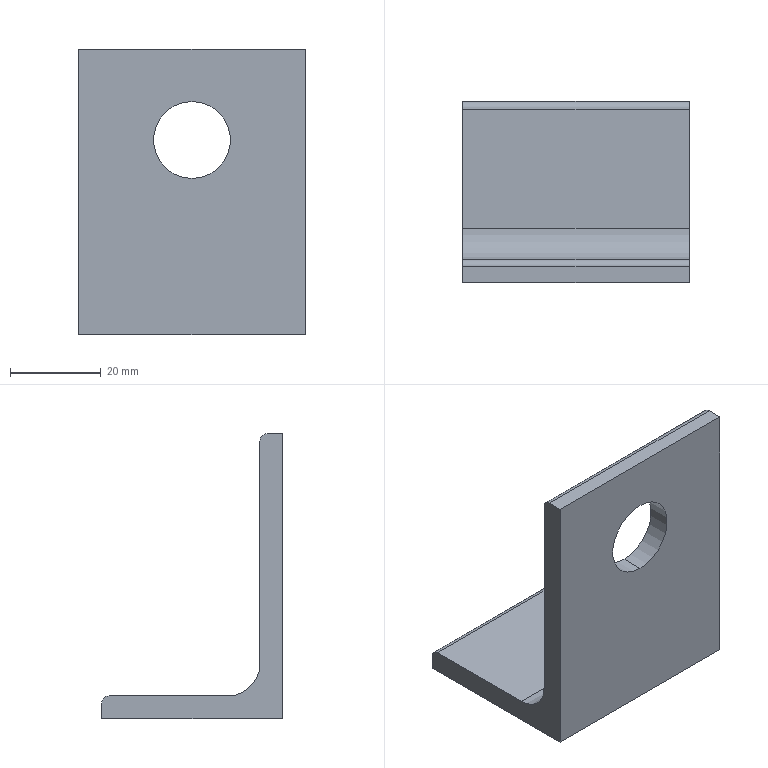Part | SolidWorks | features ICE 1, WeldMemberFeat 1, WeldmentFeature 1 | 1 solid | 13 faces | box 50 x 40 x 63 mm | volume 23831 mm3 | plane 8 | cylinder 5 | commonest cylinder face diameters 3.333 x2 17 x2 14 x1
STEP:
#1=CARTESIAN_POINT('',(25.,0.,34.5));
#2=VERTEX_POINT('',#1);
#3=CARTESIAN_POINT('',(25.,0.,51.5));
#4=VERTEX_POINT('',#3);
#5=CARTESIAN_POINT('',(25.,0.,43.));
#6=DIRECTION('',(0.,1.,0.));
#7=DIRECTION('',(0.,0.,1.));
#8=AXIS2_PLACEMENT_3D('',#5,#6,#7);
#9=CIRCLE('',#8,8.5);
#10=EDGE_CURVE('',#2,#4,#9,.T.);
#11=ORIENTED_EDGE('',*,*,#10,.F.);
#12=CARTESIAN_POINT('',(25.,5.,34.5));
#13=VERTEX_POINT('',#12);
#14=CARTESIAN_POINT('',(25.,-5.,34.5));
#15=DIRECTION('',(0.,1.,0.));
#16=VECTOR('',#15,1000.);
#17=LINE('',#14,#16);
#18=EDGE_CURVE('',#2,#13,#17,.T.);
#19=ORIENTED_EDGE('',*,*,#18,.T.);
#20=CARTESIAN_POINT('',(25.,5.,51.5));
#21=VERTEX_POINT('',#20);
#22=CARTESIAN_POINT('',(25.,5.,43.));
#23=DIRECTION('',(0.,1.,0.));
#24=DIRECTION('',(0.,0.,1.));
#25=AXIS2_PLACEMENT_3D('',#22,#23,#24);
#26=CIRCLE('',#25,8.5);
#27=EDGE_CURVE('',#13,#21,#26,.T.);
#28=ORIENTED_EDGE('',*,*,#27,.T.);
#29=CARTESIAN_POINT('',(25.,-5.,51.5));
#30=DIRECTION('',(0.,1.,0.));
#31=VECTOR('',#30,1000.);
#32=LINE('',#29,#31);
#33=EDGE_CURVE('',#4,#21,#32,.T.);
#34=ORIENTED_EDGE('',*,*,#33,.F.);
#35=EDGE_LOOP('',(#11,#19,#28,#34));
#36=FACE_OUTER_BOUND('',#35,.T.);
#37=CARTESIAN_POINT('',(25.,-5.,43.));
#38=DIRECTION('',(0.,1.,0.));
#39=DIRECTION('',(0.,0.,1.));
#40=AXIS2_PLACEMENT_3D('',#37,#38,#39);
#41=CYLINDRICAL_SURFACE('',#40,8.5);
#42=ADVANCED_FACE('',(#36),#41,.F.);
#43=CARTESIAN_POINT('',(0.,3.333,63.));
#44=VERTEX_POINT('',#43);
#45=CARTESIAN_POINT('',(0.,0.,63.));
#46=VERTEX_POINT('',#45);
#47=CARTESIAN_POINT('',(0.,0.,63.));
#48=DIRECTION('',(0.,-1.,0.));
#49=VECTOR('',#48,1000.);
#50=LINE('',#47,#49);
#51=EDGE_CURVE('',#44,#46,#50,.T.);
#52=ORIENTED_EDGE('',*,*,#51,.T.);
#53=CARTESIAN_POINT('',(50.,0.,63.));
#54=VERTEX_POINT('',#53);
#55=CARTESIAN_POINT('',(50.,0.,63.));
#56=DIRECTION('',(-1.,0.,0.));
#57=VECTOR('',#56,1000.);
#58=LINE('',#55,#57);
#59=EDGE_CURVE('',#54,#46,#58,.T.);
#60=ORIENTED_EDGE('',*,*,#59,.F.);
#61=CARTESIAN_POINT('',(50.,3.333,63.));
#62=VERTEX_POINT('',#61);
#63=CARTESIAN_POINT('',(50.,0.,63.));
#64=DIRECTION('',(0.,-1.,0.));
#65=VECTOR('',#64,1000.);
#66=LINE('',#63,#65);
#67=EDGE_CURVE('',#62,#54,#66,.T.);
#68=ORIENTED_EDGE('',*,*,#67,.F.);
#69=CARTESIAN_POINT('',(50.,3.333,63.));
#70=DIRECTION('',(-1.,0.,0.));
#71=VECTOR('',#70,1000.);
#72=LINE('',#69,#71);
#73=EDGE_CURVE('',#62,#44,#72,.T.);
#74=ORIENTED_EDGE('',*,*,#73,.T.);
#75=EDGE_LOOP('',(#52,#60,#68,#74));
#76=FACE_OUTER_BOUND('',#75,.T.);
#77=CARTESIAN_POINT('',(50.,0.,63.));
#78=DIRECTION('',(0.,0.,-1.));
#79=DIRECTION('',(0.,1.,0.));
#80=AXIS2_PLACEMENT_3D('',#77,#78,#79);
#81=PLANE('',#80);
#82=ADVANCED_FACE('',(#76),#81,.F.);
#83=CARTESIAN_POINT('',(25.,0.,43.));
#84=DIRECTION('',(0.,1.,0.));
#85=DIRECTION('',(0.,0.,1.));
#86=AXIS2_PLACEMENT_3D('',#83,#84,#85);
#87=CIRCLE('',#86,8.5);
#88=EDGE_CURVE('',#4,#2,#87,.T.);
#89=ORIENTED_EDGE('',*,*,#88,.T.);
#90=ORIENTED_EDGE('',*,*,#10,.T.);
#91=EDGE_LOOP('',(#89,#90));
#92=FACE_BOUND('',#91,.T.);
#93=CARTESIAN_POINT('',(0.,0.,0.));
#94=VERTEX_POINT('',#93);
#95=CARTESIAN_POINT('',(0.,0.,63.));
#96=DIRECTION('',(0.,0.,-1.));
#97=VECTOR('',#96,1000.);
#98=LINE('',#95,#97);
#99=EDGE_CURVE('',#46,#94,#98,.T.);
#100=ORIENTED_EDGE('',*,*,#99,.T.);
#101=CARTESIAN_POINT('',(50.,0.,0.));
#102=VERTEX_POINT('',#101);
#103=CARTESIAN_POINT('',(50.,0.,0.));
#104=DIRECTION('',(-1.,0.,0.));
#105=VECTOR('',#104,1000.);
#106=LINE('',#103,#105);
#107=EDGE_CURVE('',#102,#94,#106,.T.);
#108=ORIENTED_EDGE('',*,*,#107,.F.);
#109=CARTESIAN_POINT('',(50.,0.,63.));
#110=DIRECTION('',(0.,0.,-1.));
#111=VECTOR('',#110,1000.);
#112=LINE('',#109,#111);
#113=EDGE_CURVE('',#54,#102,#112,.T.);
#114=ORIENTED_EDGE('',*,*,#113,.F.);
#115=ORIENTED_EDGE('',*,*,#59,.T.);
#116=EDGE_LOOP('',(#100,#108,#114,#115));
#117=FACE_OUTER_BOUND('',#116,.T.);
#118=CARTESIAN_POINT('',(50.,0.,63.));
#119=DIRECTION('',(0.,1.,0.));
#120=DIRECTION('',(0.,0.,1.));
#121=AXIS2_PLACEMENT_3D('',#118,#119,#120);
#122=PLANE('',#121);
#123=ADVANCED_FACE('',(#92,#117),#122,.F.);
#124=CARTESIAN_POINT('',(0.,40.,0.));
#125=VERTEX_POINT('',#124);
#126=CARTESIAN_POINT('',(0.,0.,0.));
#127=DIRECTION('',(0.,1.,0.));
#128=VECTOR('',#127,1000.);
#129=LINE('',#126,#128);
#130=EDGE_CURVE('',#94,#125,#129,.T.);
#131=ORIENTED_EDGE('',*,*,#130,.T.);
#132=CARTESIAN_POINT('',(50.,40.,0.));
#133=VERTEX_POINT('',#132);
#134=CARTESIAN_POINT('',(50.,40.,0.));
#135=DIRECTION('',(-1.,0.,0.));
#136=VECTOR('',#135,1000.);
#137=LINE('',#134,#136);
#138=EDGE_CURVE('',#133,#125,#137,.T.);
#139=ORIENTED_EDGE('',*,*,#138,.F.);
#140=CARTESIAN_POINT('',(50.,0.,0.));
#141=DIRECTION('',(0.,1.,0.));
#142=VECTOR('',#141,1000.);
#143=LINE('',#140,#142);
#144=EDGE_CURVE('',#102,#133,#143,.T.);
#145=ORIENTED_EDGE('',*,*,#144,.F.);
#146=ORIENTED_EDGE('',*,*,#107,.T.);
#147=EDGE_LOOP('',(#131,#139,#145,#146));
#148=FACE_OUTER_BOUND('',#147,.T.);
#149=CARTESIAN_POINT('',(50.,0.,0.));
#150=DIRECTION('',(0.,0.,1.));
#151=DIRECTION('',(0.,-1.,0.));
#152=AXIS2_PLACEMENT_3D('',#149,#150,#151);
#153=PLANE('',#152);
#154=ADVANCED_FACE('',(#148),#153,.F.);
#155=CARTESIAN_POINT('',(0.,40.,3.333));
#156=VERTEX_POINT('',#155);
#157=CARTESIAN_POINT('',(0.,40.,0.));
#158=DIRECTION('',(0.,0.,1.));
#159=VECTOR('',#158,1000.);
#160=LINE('',#157,#159);
#161=EDGE_CURVE('',#125,#156,#160,.T.);
#162=ORIENTED_EDGE('',*,*,#161,.T.);
#163=CARTESIAN_POINT('',(50.,40.,3.333));
#164=VERTEX_POINT('',#163);
#165=CARTESIAN_POINT('',(50.,40.,3.333));
#166=DIRECTION('',(-1.,0.,0.));
#167=VECTOR('',#166,1000.);
#168=LINE('',#165,#167);
#169=EDGE_CURVE('',#164,#156,#168,.T.);
#170=ORIENTED_EDGE('',*,*,#169,.F.);
#171=CARTESIAN_POINT('',(50.,40.,0.));
#172=DIRECTION('',(0.,0.,1.));
#173=VECTOR('',#172,1000.);
#174=LINE('',#171,#173);
#175=EDGE_CURVE('',#133,#164,#174,.T.);
#176=ORIENTED_EDGE('',*,*,#175,.F.);
#177=ORIENTED_EDGE('',*,*,#138,.T.);
#178=EDGE_LOOP('',(#162,#170,#176,#177));
#179=FACE_OUTER_BOUND('',#178,.T.);
#180=CARTESIAN_POINT('',(50.,40.,0.));
#181=DIRECTION('',(0.,-1.,0.));
#182=DIRECTION('',(0.,0.,-1.));
#183=AXIS2_PLACEMENT_3D('',#180,#181,#182);
#184=PLANE('',#183);
#185=ADVANCED_FACE('',(#179),#184,.F.);
#186=CARTESIAN_POINT('',(0.,38.333,5.));
#187=VERTEX_POINT('',#186);
#188=CARTESIAN_POINT('',(0.,38.333,3.333));
#189=DIRECTION('',(1.,0.,0.));
#190=DIRECTION('',(0.,0.,-1.));
#191=AXIS2_PLACEMENT_3D('',#188,#189,#190);
#192=CIRCLE('',#191,1.667);
#193=EDGE_CURVE('',#156,#187,#192,.T.);
#194=ORIENTED_EDGE('',*,*,#193,.T.);
#195=CARTESIAN_POINT('',(50.,38.333,5.));
#196=VERTEX_POINT('',#195);
#197=CARTESIAN_POINT('',(50.,38.333,5.));
#198=DIRECTION('',(-1.,0.,0.));
#199=VECTOR('',#198,1000.);
#200=LINE('',#197,#199);
#201=EDGE_CURVE('',#196,#187,#200,.T.);
#202=ORIENTED_EDGE('',*,*,#201,.F.);
#203=CARTESIAN_POINT('',(50.,38.333,3.333));
#204=DIRECTION('',(1.,0.,0.));
#205=DIRECTION('',(0.,0.,-1.));
#206=AXIS2_PLACEMENT_3D('',#203,#204,#205);
#207=CIRCLE('',#206,1.667);
#208=EDGE_CURVE('',#164,#196,#207,.T.);
#209=ORIENTED_EDGE('',*,*,#208,.F.);
#210=ORIENTED_EDGE('',*,*,#169,.T.);
#211=EDGE_LOOP('',(#194,#202,#209,#210));
#212=FACE_OUTER_BOUND('',#211,.T.);
#213=CARTESIAN_POINT('',(50.,38.333,3.333));
#214=DIRECTION('',(-1.,0.,0.));
#215=DIRECTION('',(0.,0.,1.));
#216=AXIS2_PLACEMENT_3D('',#213,#214,#215);
#217=CYLINDRICAL_SURFACE('',#216,1.667);
#218=ADVANCED_FACE('',(#212),#217,.T.);
#219=CARTESIAN_POINT('',(0.,12.,5.));
#220=VERTEX_POINT('',#219);
#221=CARTESIAN_POINT('',(0.,12.,5.));
#222=DIRECTION('',(0.,-1.,0.));
#223=VECTOR('',#222,1000.);
#224=LINE('',#221,#223);
#225=EDGE_CURVE('',#187,#220,#224,.T.);
#226=ORIENTED_EDGE('',*,*,#225,.T.);
#227=CARTESIAN_POINT('',(50.,12.,5.));
#228=VERTEX_POINT('',#227);
#229=CARTESIAN_POINT('',(50.,12.,5.));
#230=DIRECTION('',(-1.,0.,0.));
#231=VECTOR('',#230,1000.);
#232=LINE('',#229,#231);
#233=EDGE_CURVE('',#228,#220,#232,.T.);
#234=ORIENTED_EDGE('',*,*,#233,.F.);
#235=CARTESIAN_POINT('',(50.,12.,5.));
#236=DIRECTION('',(0.,-1.,0.));
#237=VECTOR('',#236,1000.);
#238=LINE('',#235,#237);
#239=EDGE_CURVE('',#196,#228,#238,.T.);
#240=ORIENTED_EDGE('',*,*,#239,.F.);
#241=ORIENTED_EDGE('',*,*,#201,.T.);
#242=EDGE_LOOP('',(#226,#234,#240,#241));
#243=FACE_OUTER_BOUND('',#242,.T.);
#244=CARTESIAN_POINT('',(50.,12.,5.));
#245=DIRECTION('',(0.,0.,-1.));
#246=DIRECTION('',(0.,1.,0.));
#247=AXIS2_PLACEMENT_3D('',#244,#245,#246);
#248=PLANE('',#247);
#249=ADVANCED_FACE('',(#243),#248,.F.);
#250=CARTESIAN_POINT('',(0.,5.,12.));
#251=VERTEX_POINT('',#250);
#252=CARTESIAN_POINT('',(0.,12.,12.));
#253=DIRECTION('',(-1.,0.,0.));
#254=DIRECTION('',(0.,0.,-1.));
#255=AXIS2_PLACEMENT_3D('',#252,#253,#254);
#256=CIRCLE('',#255,7.);
#257=EDGE_CURVE('',#220,#251,#256,.T.);
#258=ORIENTED_EDGE('',*,*,#257,.T.);
#259=CARTESIAN_POINT('',(50.,5.,12.));
#260=VERTEX_POINT('',#259);
#261=CARTESIAN_POINT('',(50.,5.,12.));
#262=DIRECTION('',(-1.,0.,0.));
#263=VECTOR('',#262,1000.);
#264=LINE('',#261,#263);
#265=EDGE_CURVE('',#260,#251,#264,.T.);
#266=ORIENTED_EDGE('',*,*,#265,.F.);
#267=CARTESIAN_POINT('',(50.,12.,12.));
#268=DIRECTION('',(-1.,0.,0.));
#269=DIRECTION('',(0.,0.,-1.));
#270=AXIS2_PLACEMENT_3D('',#267,#268,#269);
#271=CIRCLE('',#270,7.);
#272=EDGE_CURVE('',#228,#260,#271,.T.);
#273=ORIENTED_EDGE('',*,*,#272,.F.);
#274=ORIENTED_EDGE('',*,*,#233,.T.);
#275=EDGE_LOOP('',(#258,#266,#273,#274));
#276=FACE_OUTER_BOUND('',#275,.T.);
#277=CARTESIAN_POINT('',(50.,12.,12.));
#278=DIRECTION('',(-1.,0.,0.));
#279=DIRECTION('',(0.,0.,1.));
#280=AXIS2_PLACEMENT_3D('',#277,#278,#279);
#281=CYLINDRICAL_SURFACE('',#280,7.);
#282=ADVANCED_FACE('',(#276),#281,.F.);
#283=CARTESIAN_POINT('',(25.,5.,43.));
#284=DIRECTION('',(0.,1.,0.));
#285=DIRECTION('',(0.,0.,1.));
#286=AXIS2_PLACEMENT_3D('',#283,#284,#285);
#287=CIRCLE('',#286,8.5);
#288=EDGE_CURVE('',#21,#13,#287,.T.);
#289=ORIENTED_EDGE('',*,*,#288,.F.);
#290=ORIENTED_EDGE('',*,*,#27,.F.);
#291=EDGE_LOOP('',(#289,#290));
#292=FACE_BOUND('',#291,.T.);
#293=CARTESIAN_POINT('',(0.,5.,61.333));
#294=VERTEX_POINT('',#293);
#295=CARTESIAN_POINT('',(0.,5.,61.333));
#296=DIRECTION('',(0.,0.,1.));
#297=VECTOR('',#296,1000.);
#298=LINE('',#295,#297);
#299=EDGE_CURVE('',#251,#294,#298,.T.);
#300=ORIENTED_EDGE('',*,*,#299,.T.);
#301=CARTESIAN_POINT('',(50.,5.,61.333));
#302=VERTEX_POINT('',#301);
#303=CARTESIAN_POINT('',(50.,5.,61.333));
#304=DIRECTION('',(-1.,0.,0.));
#305=VECTOR('',#304,1000.);
#306=LINE('',#303,#305);
#307=EDGE_CURVE('',#302,#294,#306,.T.);
#308=ORIENTED_EDGE('',*,*,#307,.F.);
#309=CARTESIAN_POINT('',(50.,5.,61.333));
#310=DIRECTION('',(0.,0.,1.));
#311=VECTOR('',#310,1000.);
#312=LINE('',#309,#311);
#313=EDGE_CURVE('',#260,#302,#312,.T.);
#314=ORIENTED_EDGE('',*,*,#313,.F.);
#315=ORIENTED_EDGE('',*,*,#265,.T.);
#316=EDGE_LOOP('',(#300,#308,#314,#315));
#317=FACE_OUTER_BOUND('',#316,.T.);
#318=CARTESIAN_POINT('',(50.,5.,61.333));
#319=DIRECTION('',(0.,-1.,0.));
#320=DIRECTION('',(0.,0.,-1.));
#321=AXIS2_PLACEMENT_3D('',#318,#319,#320);
#322=PLANE('',#321);
#323=ADVANCED_FACE('',(#292,#317),#322,.F.);
#324=CARTESIAN_POINT('',(0.,3.333,61.333));
#325=DIRECTION('',(1.,0.,0.));
#326=DIRECTION('',(0.,0.,1.));
#327=AXIS2_PLACEMENT_3D('',#324,#325,#326);
#328=CIRCLE('',#327,1.667);
#329=EDGE_CURVE('',#294,#44,#328,.T.);
#330=ORIENTED_EDGE('',*,*,#329,.T.);
#331=ORIENTED_EDGE('',*,*,#73,.F.);
#332=CARTESIAN_POINT('',(50.,3.333,61.333));
#333=DIRECTION('',(1.,0.,0.));
#334=DIRECTION('',(0.,0.,1.));
#335=AXIS2_PLACEMENT_3D('',#332,#333,#334);
#336=CIRCLE('',#335,1.667);
#337=EDGE_CURVE('',#302,#62,#336,.T.);
#338=ORIENTED_EDGE('',*,*,#337,.F.);
#339=ORIENTED_EDGE('',*,*,#307,.T.);
#340=EDGE_LOOP('',(#330,#331,#338,#339));
#341=FACE_OUTER_BOUND('',#340,.T.);
#342=CARTESIAN_POINT('',(50.,3.333,61.333));
#343=DIRECTION('',(-1.,0.,0.));
#344=DIRECTION('',(0.,0.,1.));
#345=AXIS2_PLACEMENT_3D('',#342,#343,#344);
#346=CYLINDRICAL_SURFACE('',#345,1.667);
#347=ADVANCED_FACE('',(#341),#346,.T.);
#348=ORIENTED_EDGE('',*,*,#67,.T.);
#349=ORIENTED_EDGE('',*,*,#113,.T.);
#350=ORIENTED_EDGE('',*,*,#144,.T.);
#351=ORIENTED_EDGE('',*,*,#175,.T.);
#352=ORIENTED_EDGE('',*,*,#208,.T.);
#353=ORIENTED_EDGE('',*,*,#239,.T.);
#354=ORIENTED_EDGE('',*,*,#272,.T.);
#355=ORIENTED_EDGE('',*,*,#313,.T.);
#356=ORIENTED_EDGE('',*,*,#337,.T.);
#357=EDGE_LOOP('',(#348,#349,#350,#351,#352,#353,#354,#355,#356));
#358=FACE_OUTER_BOUND('',#357,.T.);
#359=CARTESIAN_POINT('',(50.,3.333,61.333));
#360=DIRECTION('',(-1.,0.,0.));
#361=DIRECTION('',(0.,0.,1.));
#362=AXIS2_PLACEMENT_3D('',#359,#360,#361);
#363=PLANE('',#362);
#364=ADVANCED_FACE('',(#358),#363,.F.);
#365=ORIENTED_EDGE('',*,*,#51,.F.);
#366=ORIENTED_EDGE('',*,*,#329,.F.);
#367=ORIENTED_EDGE('',*,*,#299,.F.);
#368=ORIENTED_EDGE('',*,*,#257,.F.);
#369=ORIENTED_EDGE('',*,*,#225,.F.);
#370=ORIENTED_EDGE('',*,*,#193,.F.);
#371=ORIENTED_EDGE('',*,*,#161,.F.);
#372=ORIENTED_EDGE('',*,*,#130,.F.);
#373=ORIENTED_EDGE('',*,*,#99,.F.);
#374=EDGE_LOOP('',(#365,#366,#367,#368,#369,#370,#371,#372,#373));
#375=FACE_OUTER_BOUND('',#374,.T.);
#376=CARTESIAN_POINT('',(0.,3.333,61.333));
#377=DIRECTION('',(-1.,0.,0.));
#378=DIRECTION('',(0.,0.,1.));
#379=AXIS2_PLACEMENT_3D('',#376,#377,#378);
#380=PLANE('',#379);
#381=ADVANCED_FACE('',(#375),#380,.T.);
#382=ORIENTED_EDGE('',*,*,#18,.F.);
#383=ORIENTED_EDGE('',*,*,#88,.F.);
#384=ORIENTED_EDGE('',*,*,#33,.T.);
#385=ORIENTED_EDGE('',*,*,#288,.T.);
#386=EDGE_LOOP('',(#382,#383,#384,#385));
#387=FACE_OUTER_BOUND('',#386,.T.);
#388=CARTESIAN_POINT('',(25.,-5.,43.));
#389=DIRECTION('',(0.,1.,0.));
#390=DIRECTION('',(0.,0.,1.));
#391=AXIS2_PLACEMENT_3D('',#388,#389,#390);
#392=CYLINDRICAL_SURFACE('',#391,8.5);
#393=ADVANCED_FACE('',(#387),#392,.F.);
#394=CLOSED_SHELL('',(#42,#82,#123,#154,#185,#218,#249,#282,#323,#347,#364,#381,#393));
#395=MANIFOLD_SOLID_BREP('',#394);
#396=CARTESIAN_POINT('',(0.,0.,0.));
#397=DIRECTION('',(0.,0.,1.));
#398=DIRECTION('',(1.,0.,0.));
#399=AXIS2_PLACEMENT_3D('',#396,#397,#398);
#400=(LENGTH_UNIT()NAMED_UNIT(*)SI_UNIT(.MILLI.,.METRE.));
#401=UNCERTAINTY_MEASURE_WITH_UNIT(LENGTH_MEASURE(0.00001),#400,'','');
#402=(NAMED_UNIT(*)PLANE_ANGLE_UNIT()SI_UNIT($,.RADIAN.));
#403=(NAMED_UNIT(*)SI_UNIT($,.STERADIAN.)SOLID_ANGLE_UNIT());
#404=(GEOMETRIC_REPRESENTATION_CONTEXT(3)GLOBAL_UNCERTAINTY_ASSIGNED_CONTEXT((#401))GLOBAL_UNIT_ASSIGNED_CONTEXT((#400,#402,#403))REPRESENTATION_CONTEXT('',''));
#405=ADVANCED_BREP_SHAPE_REPRESENTATION('',(#395,#399),#404);